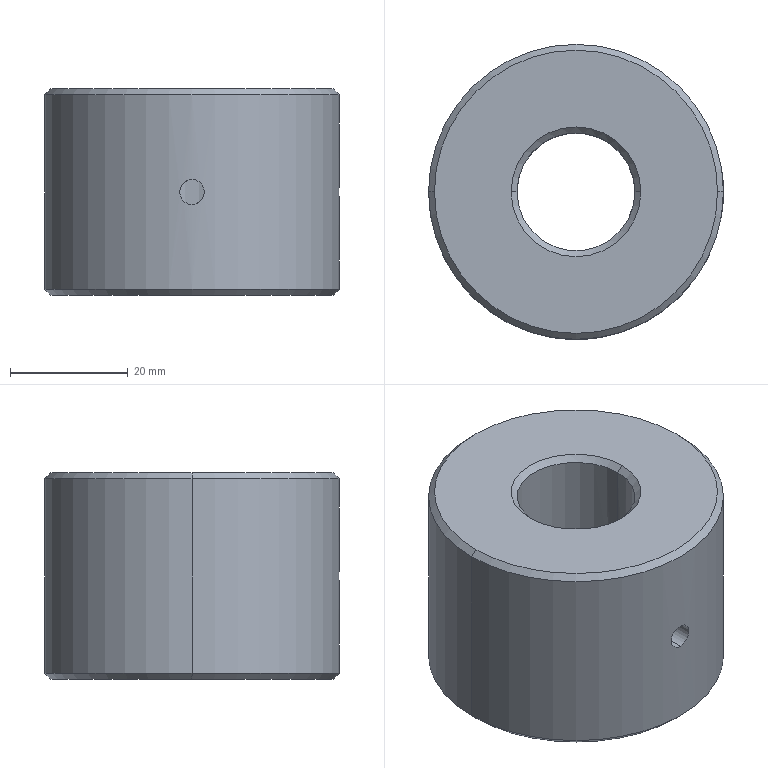Part | SolidWorks | features BaseBody 1 | 1 solid | 18 faces | box 50 x 50 x 35 mm | volume 57090 mm3 | cylinder 8 | cone 8 | plane 2 | commonest cylinder face diameters 4.2 x4 20 x2 50 x2
STEP:
#1=CARTESIAN_POINT('',(0.,-10.,15.4));
#2=VERTEX_POINT('',#1);
#3=CARTESIAN_POINT('',(0.,-10.,19.6));
#4=VERTEX_POINT('',#3);
#5=CARTESIAN_POINT('',(0.,-10.,15.4));
#6=CARTESIAN_POINT('',(-0.1391,-10.,15.4));
#7=CARTESIAN_POINT('',(-0.2759,-9.997,15.414));
#8=CARTESIAN_POINT('',(-0.5447,-9.986,15.467));
#9=CARTESIAN_POINT('',(-0.6783,-9.978,15.508));
#10=CARTESIAN_POINT('',(-0.9324,-9.957,15.613));
#11=CARTESIAN_POINT('',(-1.053,-9.945,15.678));
#12=CARTESIAN_POINT('',(-1.281,-9.918,15.83));
#13=CARTESIAN_POINT('',(-1.388,-9.904,15.919));
#14=CARTESIAN_POINT('',(-1.678,-9.86,16.208));
#15=CARTESIAN_POINT('',(-1.834,-9.831,16.442));
#16=CARTESIAN_POINT('',(-1.992,-9.8,16.821));
#17=CARTESIAN_POINT('',(-2.032,-9.791,16.953));
#18=CARTESIAN_POINT('',(-2.086,-9.78,17.224));
#19=CARTESIAN_POINT('',(-2.1,-9.777,17.361));
#20=CARTESIAN_POINT('',(-2.1,-9.777,17.636));
#21=CARTESIAN_POINT('',(-2.086,-9.78,17.775));
#22=CARTESIAN_POINT('',(-2.033,-9.791,18.045));
#23=CARTESIAN_POINT('',(-1.993,-9.8,18.176));
#24=CARTESIAN_POINT('',(-1.835,-9.831,18.558));
#25=CARTESIAN_POINT('',(-1.681,-9.86,18.789));
#26=CARTESIAN_POINT('',(-1.388,-9.904,19.082));
#27=CARTESIAN_POINT('',(-1.283,-9.918,19.168));
#28=CARTESIAN_POINT('',(-1.056,-9.945,19.32));
#29=CARTESIAN_POINT('',(-0.9328,-9.957,19.386));
#30=CARTESIAN_POINT('',(-0.6792,-9.978,19.492));
#31=CARTESIAN_POINT('',(-0.5483,-9.986,19.532));
#32=CARTESIAN_POINT('',(-0.2784,-9.997,19.586));
#33=CARTESIAN_POINT('',(-0.1391,-10.,19.6));
#34=CARTESIAN_POINT('',(0.,-10.,19.6));
#35=B_SPLINE_CURVE_WITH_KNOTS('',3,(#5,#6,#7,#8,#9,#10,#11,#12,#13,#14,#15,#16,#17,#18,#19,#20,#21,#22,#23,#24,#25,#26,#27,#28,#29,#30,#31,#32,#33,#34),.UNSPECIFIED.,.F.,.F.,(4,2,2,2,2,2,2,2,2,2,2,2,2,2,4),(0.,0.0004114,0.0008228,0.001234,0.001646,0.002468,0.00288,0.003291,0.003702,0.004114,0.004937,0.005348,0.005759,0.006171,0.006582),.UNSPECIFIED.);
#36=EDGE_CURVE('',#2,#4,#35,.T.);
#37=ORIENTED_EDGE('',*,*,#36,.T.);
#38=CARTESIAN_POINT('',(0.,-25.,19.6));
#39=VERTEX_POINT('',#38);
#40=CARTESIAN_POINT('',(0.,-25.,19.6));
#41=DIRECTION('',(0.,-1.,0.));
#42=VECTOR('',#41,1000.);
#43=LINE('',#40,#42);
#44=EDGE_CURVE('',#4,#39,#43,.T.);
#45=ORIENTED_EDGE('',*,*,#44,.T.);
#46=CARTESIAN_POINT('',(0.,-25.,15.4));
#47=VERTEX_POINT('',#46);
#48=CARTESIAN_POINT('',(0.,-25.,15.4));
#49=CARTESIAN_POINT('',(-0.1388,-25.,15.4));
#50=CARTESIAN_POINT('',(-0.2752,-24.999,15.414));
#51=CARTESIAN_POINT('',(-0.5437,-24.994,15.467));
#52=CARTESIAN_POINT('',(-0.6771,-24.991,15.507));
#53=CARTESIAN_POINT('',(-0.9313,-24.983,15.613));
#54=CARTESIAN_POINT('',(-1.052,-24.978,15.677));
#55=CARTESIAN_POINT('',(-1.28,-24.967,15.83));
#56=CARTESIAN_POINT('',(-1.388,-24.962,15.918));
#57=CARTESIAN_POINT('',(-1.679,-24.944,16.209));
#58=CARTESIAN_POINT('',(-1.835,-24.933,16.443));
#59=CARTESIAN_POINT('',(-2.045,-24.916,16.948));
#60=CARTESIAN_POINT('',(-2.1,-24.912,17.225));
#61=CARTESIAN_POINT('',(-2.1,-24.912,17.636));
#62=CARTESIAN_POINT('',(-2.086,-24.913,17.775));
#63=CARTESIAN_POINT('',(-2.033,-24.917,18.044));
#64=CARTESIAN_POINT('',(-1.993,-24.92,18.175));
#65=CARTESIAN_POINT('',(-1.888,-24.929,18.429));
#66=CARTESIAN_POINT('',(-1.823,-24.934,18.552));
#67=CARTESIAN_POINT('',(-1.671,-24.944,18.78));
#68=CARTESIAN_POINT('',(-1.584,-24.95,18.886));
#69=CARTESIAN_POINT('',(-1.388,-24.962,19.082));
#70=CARTESIAN_POINT('',(-1.282,-24.967,19.169));
#71=CARTESIAN_POINT('',(-1.055,-24.978,19.321));
#72=CARTESIAN_POINT('',(-0.932,-24.983,19.387));
#73=CARTESIAN_POINT('',(-0.6777,-24.991,19.492));
#74=CARTESIAN_POINT('',(-0.5468,-24.994,19.532));
#75=CARTESIAN_POINT('',(-0.2777,-24.999,19.586));
#76=CARTESIAN_POINT('',(-0.1388,-25.,19.6));
#77=CARTESIAN_POINT('',(0.,-25.,19.6));
#78=B_SPLINE_CURVE_WITH_KNOTS('',3,(#48,#49,#50,#51,#52,#53,#54,#55,#56,#57,#58,#59,#60,#61,#62,#63,#64,#65,#66,#67,#68,#69,#70,#71,#72,#73,#74,#75,#76,#77),.UNSPECIFIED.,.F.,.F.,(4,2,2,2,2,2,2,2,2,2,2,2,2,2,4),(0.,0.0004104,0.0008209,0.001231,0.001642,0.002463,0.003284,0.003694,0.004104,0.004515,0.004925,0.005336,0.005746,0.006157,0.006567),.UNSPECIFIED.);
#79=EDGE_CURVE('',#47,#39,#78,.T.);
#80=ORIENTED_EDGE('',*,*,#79,.F.);
#81=CARTESIAN_POINT('',(0.,-25.,15.4));
#82=DIRECTION('',(0.,-1.,0.));
#83=VECTOR('',#82,1000.);
#84=LINE('',#81,#83);
#85=EDGE_CURVE('',#2,#47,#84,.T.);
#86=ORIENTED_EDGE('',*,*,#85,.F.);
#87=EDGE_LOOP('',(#37,#45,#80,#86));
#88=FACE_OUTER_BOUND('',#87,.T.);
#89=CARTESIAN_POINT('',(0.,-25.,17.5));
#90=DIRECTION('',(0.,-1.,0.));
#91=DIRECTION('',(0.,0.,-1.));
#92=AXIS2_PLACEMENT_3D('',#89,#90,#91);
#93=CYLINDRICAL_SURFACE('',#92,2.1);
#94=ADVANCED_FACE('',(#88),#93,.F.);
#95=CARTESIAN_POINT('',(10.,0.,15.4));
#96=VERTEX_POINT('',#95);
#97=CARTESIAN_POINT('',(10.,0.,19.6));
#98=VERTEX_POINT('',#97);
#99=CARTESIAN_POINT('',(10.,0.,15.4));
#100=CARTESIAN_POINT('',(10.,-0.1391,15.4));
#101=CARTESIAN_POINT('',(9.997,-0.2759,15.414));
#102=CARTESIAN_POINT('',(9.986,-0.5447,15.467));
#103=CARTESIAN_POINT('',(9.978,-0.6783,15.508));
#104=CARTESIAN_POINT('',(9.957,-0.9324,15.613));
#105=CARTESIAN_POINT('',(9.945,-1.053,15.678));
#106=CARTESIAN_POINT('',(9.918,-1.281,15.83));
#107=CARTESIAN_POINT('',(9.904,-1.388,15.919));
#108=CARTESIAN_POINT('',(9.86,-1.678,16.208));
#109=CARTESIAN_POINT('',(9.831,-1.834,16.442));
#110=CARTESIAN_POINT('',(9.8,-1.992,16.821));
#111=CARTESIAN_POINT('',(9.791,-2.032,16.953));
#112=CARTESIAN_POINT('',(9.78,-2.086,17.224));
#113=CARTESIAN_POINT('',(9.777,-2.1,17.361));
#114=CARTESIAN_POINT('',(9.777,-2.1,17.636));
#115=CARTESIAN_POINT('',(9.78,-2.086,17.775));
#116=CARTESIAN_POINT('',(9.791,-2.033,18.045));
#117=CARTESIAN_POINT('',(9.8,-1.993,18.176));
#118=CARTESIAN_POINT('',(9.831,-1.835,18.558));
#119=CARTESIAN_POINT('',(9.86,-1.681,18.789));
#120=CARTESIAN_POINT('',(9.904,-1.388,19.082));
#121=CARTESIAN_POINT('',(9.918,-1.283,19.168));
#122=CARTESIAN_POINT('',(9.945,-1.056,19.32));
#123=CARTESIAN_POINT('',(9.957,-0.9328,19.386));
#124=CARTESIAN_POINT('',(9.978,-0.6792,19.492));
#125=CARTESIAN_POINT('',(9.986,-0.5483,19.532));
#126=CARTESIAN_POINT('',(9.997,-0.2784,19.586));
#127=CARTESIAN_POINT('',(10.,-0.1391,19.6));
#128=CARTESIAN_POINT('',(10.,0.,19.6));
#129=B_SPLINE_CURVE_WITH_KNOTS('',3,(#99,#100,#101,#102,#103,#104,#105,#106,#107,#108,#109,#110,#111,#112,#113,#114,#115,#116,#117,#118,#119,#120,#121,#122,#123,#124,#125,#126,#127,#128),.UNSPECIFIED.,.F.,.F.,(4,2,2,2,2,2,2,2,2,2,2,2,2,2,4),(0.,0.0004114,0.0008228,0.001234,0.001646,0.002468,0.00288,0.003291,0.003702,0.004114,0.004937,0.005348,0.005759,0.006171,0.006582),.UNSPECIFIED.);
#130=EDGE_CURVE('',#96,#98,#129,.T.);
#131=ORIENTED_EDGE('',*,*,#130,.T.);
#132=CARTESIAN_POINT('',(25.,0.,19.6));
#133=VERTEX_POINT('',#132);
#134=CARTESIAN_POINT('',(25.,0.,19.6));
#135=DIRECTION('',(1.,0.,0.));
#136=VECTOR('',#135,1000.);
#137=LINE('',#134,#136);
#138=EDGE_CURVE('',#98,#133,#137,.T.);
#139=ORIENTED_EDGE('',*,*,#138,.T.);
#140=CARTESIAN_POINT('',(25.,0.,15.4));
#141=VERTEX_POINT('',#140);
#142=CARTESIAN_POINT('',(25.,0.,15.4));
#143=CARTESIAN_POINT('',(25.,-0.1388,15.4));
#144=CARTESIAN_POINT('',(24.999,-0.2752,15.414));
#145=CARTESIAN_POINT('',(24.994,-0.5437,15.467));
#146=CARTESIAN_POINT('',(24.991,-0.6771,15.507));
#147=CARTESIAN_POINT('',(24.983,-0.9313,15.613));
#148=CARTESIAN_POINT('',(24.978,-1.052,15.677));
#149=CARTESIAN_POINT('',(24.967,-1.28,15.83));
#150=CARTESIAN_POINT('',(24.962,-1.388,15.918));
#151=CARTESIAN_POINT('',(24.944,-1.679,16.209));
#152=CARTESIAN_POINT('',(24.933,-1.835,16.443));
#153=CARTESIAN_POINT('',(24.916,-2.045,16.948));
#154=CARTESIAN_POINT('',(24.912,-2.1,17.225));
#155=CARTESIAN_POINT('',(24.912,-2.1,17.636));
#156=CARTESIAN_POINT('',(24.913,-2.086,17.775));
#157=CARTESIAN_POINT('',(24.917,-2.033,18.044));
#158=CARTESIAN_POINT('',(24.92,-1.993,18.175));
#159=CARTESIAN_POINT('',(24.929,-1.888,18.429));
#160=CARTESIAN_POINT('',(24.934,-1.823,18.552));
#161=CARTESIAN_POINT('',(24.944,-1.671,18.78));
#162=CARTESIAN_POINT('',(24.95,-1.584,18.886));
#163=CARTESIAN_POINT('',(24.962,-1.388,19.082));
#164=CARTESIAN_POINT('',(24.967,-1.282,19.169));
#165=CARTESIAN_POINT('',(24.978,-1.055,19.321));
#166=CARTESIAN_POINT('',(24.983,-0.932,19.387));
#167=CARTESIAN_POINT('',(24.991,-0.6777,19.492));
#168=CARTESIAN_POINT('',(24.994,-0.5468,19.532));
#169=CARTESIAN_POINT('',(24.999,-0.2777,19.586));
#170=CARTESIAN_POINT('',(25.,-0.1388,19.6));
#171=CARTESIAN_POINT('',(25.,0.,19.6));
#172=B_SPLINE_CURVE_WITH_KNOTS('',3,(#142,#143,#144,#145,#146,#147,#148,#149,#150,#151,#152,#153,#154,#155,#156,#157,#158,#159,#160,#161,#162,#163,#164,#165,#166,#167,#168,#169,#170,#171),.UNSPECIFIED.,.F.,.F.,(4,2,2,2,2,2,2,2,2,2,2,2,2,2,4),(0.,0.0004104,0.0008209,0.001231,0.001642,0.002463,0.003284,0.003694,0.004104,0.004515,0.004925,0.005336,0.005746,0.006157,0.006567),.UNSPECIFIED.);
#173=EDGE_CURVE('',#141,#133,#172,.T.);
#174=ORIENTED_EDGE('',*,*,#173,.F.);
#175=CARTESIAN_POINT('',(25.,0.,15.4));
#176=DIRECTION('',(1.,0.,0.));
#177=VECTOR('',#176,1000.);
#178=LINE('',#175,#177);
#179=EDGE_CURVE('',#96,#141,#178,.T.);
#180=ORIENTED_EDGE('',*,*,#179,.F.);
#181=EDGE_LOOP('',(#131,#139,#174,#180));
#182=FACE_OUTER_BOUND('',#181,.T.);
#183=CARTESIAN_POINT('',(25.,0.,17.5));
#184=DIRECTION('',(1.,0.,0.));
#185=DIRECTION('',(0.,0.,-1.));
#186=AXIS2_PLACEMENT_3D('',#183,#184,#185);
#187=CYLINDRICAL_SURFACE('',#186,2.1);
#188=ADVANCED_FACE('',(#182),#187,.F.);
#189=CARTESIAN_POINT('',(10.,0.,1.));
#190=VERTEX_POINT('',#189);
#191=CARTESIAN_POINT('',(-10.,0.,1.));
#192=VERTEX_POINT('',#191);
#193=CARTESIAN_POINT('',(0.,0.,1.));
#194=DIRECTION('',(0.,0.,-1.));
#195=DIRECTION('',(1.,0.,0.));
#196=AXIS2_PLACEMENT_3D('',#193,#194,#195);
#197=CIRCLE('',#196,10.);
#198=EDGE_CURVE('',#190,#192,#197,.T.);
#199=ORIENTED_EDGE('',*,*,#198,.F.);
#200=CARTESIAN_POINT('',(11.,0.,0.));
#201=VERTEX_POINT('',#200);
#202=CARTESIAN_POINT('',(11.,0.,0.));
#203=DIRECTION('',(0.7071,0.,-0.7071));
#204=VECTOR('',#203,1000.);
#205=LINE('',#202,#204);
#206=EDGE_CURVE('',#190,#201,#205,.T.);
#207=ORIENTED_EDGE('',*,*,#206,.T.);
#208=CARTESIAN_POINT('',(-11.,0.,0.));
#209=VERTEX_POINT('',#208);
#210=CARTESIAN_POINT('',(0.,0.,0.));
#211=DIRECTION('',(0.,0.,1.));
#212=DIRECTION('',(1.,0.,0.));
#213=AXIS2_PLACEMENT_3D('',#210,#211,#212);
#214=CIRCLE('',#213,11.);
#215=EDGE_CURVE('',#209,#201,#214,.T.);
#216=ORIENTED_EDGE('',*,*,#215,.F.);
#217=CARTESIAN_POINT('',(-11.,0.,0.));
#218=DIRECTION('',(-0.7071,0.,-0.7071));
#219=VECTOR('',#218,1000.);
#220=LINE('',#217,#219);
#221=EDGE_CURVE('',#192,#209,#220,.T.);
#222=ORIENTED_EDGE('',*,*,#221,.F.);
#223=EDGE_LOOP('',(#199,#207,#216,#222));
#224=FACE_OUTER_BOUND('',#223,.T.);
#225=CARTESIAN_POINT('',(0.,0.,0.));
#226=DIRECTION('',(0.,0.,-1.));
#227=DIRECTION('',(-1.,0.,0.));
#228=AXIS2_PLACEMENT_3D('',#225,#226,#227);
#229=CONICAL_SURFACE('',#228,11.,0.7854);
#230=ADVANCED_FACE('',(#224),#229,.F.);
#231=CARTESIAN_POINT('',(-10.,0.,34.));
#232=VERTEX_POINT('',#231);
#233=CARTESIAN_POINT('',(10.,0.,34.));
#234=VERTEX_POINT('',#233);
#235=CARTESIAN_POINT('',(0.,0.,34.));
#236=DIRECTION('',(0.,0.,1.));
#237=DIRECTION('',(1.,0.,0.));
#238=AXIS2_PLACEMENT_3D('',#235,#236,#237);
#239=CIRCLE('',#238,10.);
#240=EDGE_CURVE('',#232,#234,#239,.T.);
#241=ORIENTED_EDGE('',*,*,#240,.F.);
#242=CARTESIAN_POINT('',(-11.,0.,35.));
#243=VERTEX_POINT('',#242);
#244=CARTESIAN_POINT('',(-10.,0.,34.));
#245=DIRECTION('',(-0.7071,0.,0.7071));
#246=VECTOR('',#245,1000.);
#247=LINE('',#244,#246);
#248=EDGE_CURVE('',#232,#243,#247,.T.);
#249=ORIENTED_EDGE('',*,*,#248,.T.);
#250=CARTESIAN_POINT('',(11.,0.,35.));
#251=VERTEX_POINT('',#250);
#252=CARTESIAN_POINT('',(0.,0.,35.));
#253=DIRECTION('',(0.,0.,-1.));
#254=DIRECTION('',(1.,0.,0.));
#255=AXIS2_PLACEMENT_3D('',#252,#253,#254);
#256=CIRCLE('',#255,11.);
#257=EDGE_CURVE('',#251,#243,#256,.T.);
#258=ORIENTED_EDGE('',*,*,#257,.F.);
#259=CARTESIAN_POINT('',(10.,0.,34.));
#260=DIRECTION('',(0.7071,0.,0.7071));
#261=VECTOR('',#260,1000.);
#262=LINE('',#259,#261);
#263=EDGE_CURVE('',#234,#251,#262,.T.);
#264=ORIENTED_EDGE('',*,*,#263,.F.);
#265=EDGE_LOOP('',(#241,#249,#258,#264));
#266=FACE_OUTER_BOUND('',#265,.T.);
#267=CARTESIAN_POINT('',(0.,0.,34.));
#268=DIRECTION('',(0.,0.,1.));
#269=DIRECTION('',(1.,0.,0.));
#270=AXIS2_PLACEMENT_3D('',#267,#268,#269);
#271=CONICAL_SURFACE('',#270,10.,0.7854);
#272=ADVANCED_FACE('',(#266),#271,.F.);
#273=CARTESIAN_POINT('',(24.,0.,35.));
#274=VERTEX_POINT('',#273);
#275=CARTESIAN_POINT('',(-24.,0.,35.));
#276=VERTEX_POINT('',#275);
#277=CARTESIAN_POINT('',(0.,0.,35.));
#278=DIRECTION('',(0.,0.,1.));
#279=DIRECTION('',(1.,0.,0.));
#280=AXIS2_PLACEMENT_3D('',#277,#278,#279);
#281=CIRCLE('',#280,24.);
#282=EDGE_CURVE('',#274,#276,#281,.T.);
#283=ORIENTED_EDGE('',*,*,#282,.F.);
#284=CARTESIAN_POINT('',(25.,0.,34.));
#285=VERTEX_POINT('',#284);
#286=CARTESIAN_POINT('',(24.,0.,35.));
#287=DIRECTION('',(0.7071,0.,-0.7071));
#288=VECTOR('',#287,1000.);
#289=LINE('',#286,#288);
#290=EDGE_CURVE('',#274,#285,#289,.T.);
#291=ORIENTED_EDGE('',*,*,#290,.T.);
#292=CARTESIAN_POINT('',(-25.,0.,34.));
#293=VERTEX_POINT('',#292);
#294=CARTESIAN_POINT('',(0.,0.,34.));
#295=DIRECTION('',(0.,0.,-1.));
#296=DIRECTION('',(1.,0.,0.));
#297=AXIS2_PLACEMENT_3D('',#294,#295,#296);
#298=CIRCLE('',#297,25.);
#299=EDGE_CURVE('',#293,#285,#298,.T.);
#300=ORIENTED_EDGE('',*,*,#299,.F.);
#301=CARTESIAN_POINT('',(-24.,0.,35.));
#302=DIRECTION('',(-0.7071,0.,-0.7071));
#303=VECTOR('',#302,1000.);
#304=LINE('',#301,#303);
#305=EDGE_CURVE('',#276,#293,#304,.T.);
#306=ORIENTED_EDGE('',*,*,#305,.F.);
#307=EDGE_LOOP('',(#283,#291,#300,#306));
#308=FACE_OUTER_BOUND('',#307,.T.);
#309=CARTESIAN_POINT('',(0.,0.,35.));
#310=DIRECTION('',(0.,0.,-1.));
#311=DIRECTION('',(-1.,0.,0.));
#312=AXIS2_PLACEMENT_3D('',#309,#310,#311);
#313=CONICAL_SURFACE('',#312,24.,0.7854);
#314=ADVANCED_FACE('',(#308),#313,.T.);
#315=CARTESIAN_POINT('',(-24.,0.,0.));
#316=VERTEX_POINT('',#315);
#317=CARTESIAN_POINT('',(24.,0.,0.));
#318=VERTEX_POINT('',#317);
#319=CARTESIAN_POINT('',(0.,0.,0.));
#320=DIRECTION('',(0.,0.,-1.));
#321=DIRECTION('',(1.,0.,0.));
#322=AXIS2_PLACEMENT_3D('',#319,#320,#321);
#323=CIRCLE('',#322,24.);
#324=EDGE_CURVE('',#316,#318,#323,.T.);
#325=ORIENTED_EDGE('',*,*,#324,.F.);
#326=CARTESIAN_POINT('',(-25.,0.,1.));
#327=VERTEX_POINT('',#326);
#328=CARTESIAN_POINT('',(-25.,0.,1.));
#329=DIRECTION('',(-0.7071,0.,0.7071));
#330=VECTOR('',#329,1000.);
#331=LINE('',#328,#330);
#332=EDGE_CURVE('',#316,#327,#331,.T.);
#333=ORIENTED_EDGE('',*,*,#332,.T.);
#334=CARTESIAN_POINT('',(25.,0.,1.));
#335=VERTEX_POINT('',#334);
#336=CARTESIAN_POINT('',(0.,0.,1.));
#337=DIRECTION('',(0.,0.,1.));
#338=DIRECTION('',(1.,0.,0.));
#339=AXIS2_PLACEMENT_3D('',#336,#337,#338);
#340=CIRCLE('',#339,25.);
#341=EDGE_CURVE('',#335,#327,#340,.T.);
#342=ORIENTED_EDGE('',*,*,#341,.F.);
#343=CARTESIAN_POINT('',(25.,0.,1.));
#344=DIRECTION('',(0.7071,0.,0.7071));
#345=VECTOR('',#344,1000.);
#346=LINE('',#343,#345);
#347=EDGE_CURVE('',#318,#335,#346,.T.);
#348=ORIENTED_EDGE('',*,*,#347,.F.);
#349=EDGE_LOOP('',(#325,#333,#342,#348));
#350=FACE_OUTER_BOUND('',#349,.T.);
#351=CARTESIAN_POINT('',(0.,0.,1.));
#352=DIRECTION('',(0.,0.,1.));
#353=DIRECTION('',(1.,0.,0.));
#354=AXIS2_PLACEMENT_3D('',#351,#352,#353);
#355=CONICAL_SURFACE('',#354,25.,0.7854);
#356=ADVANCED_FACE('',(#350),#355,.T.);
#357=ORIENTED_EDGE('',*,*,#36,.F.);
#358=CARTESIAN_POINT('',(0.,-10.,19.6));
#359=CARTESIAN_POINT('',(0.1391,-10.,19.6));
#360=CARTESIAN_POINT('',(0.2759,-9.997,19.586));
#361=CARTESIAN_POINT('',(0.5447,-9.986,19.533));
#362=CARTESIAN_POINT('',(0.6783,-9.978,19.492));
#363=CARTESIAN_POINT('',(0.9324,-9.957,19.387));
#364=CARTESIAN_POINT('',(1.053,-9.945,19.322));
#365=CARTESIAN_POINT('',(1.281,-9.918,19.17));
#366=CARTESIAN_POINT('',(1.388,-9.904,19.081));
#367=CARTESIAN_POINT('',(1.678,-9.86,18.792));
#368=CARTESIAN_POINT('',(1.834,-9.831,18.558));
#369=CARTESIAN_POINT('',(1.992,-9.8,18.179));
#370=CARTESIAN_POINT('',(2.032,-9.791,18.047));
#371=CARTESIAN_POINT('',(2.086,-9.78,17.776));
#372=CARTESIAN_POINT('',(2.1,-9.777,17.639));
#373=CARTESIAN_POINT('',(2.1,-9.777,17.364));
#374=CARTESIAN_POINT('',(2.086,-9.78,17.225));
#375=CARTESIAN_POINT('',(2.033,-9.791,16.955));
#376=CARTESIAN_POINT('',(1.993,-9.8,16.824));
#377=CARTESIAN_POINT('',(1.835,-9.831,16.442));
#378=CARTESIAN_POINT('',(1.681,-9.86,16.211));
#379=CARTESIAN_POINT('',(1.388,-9.904,15.918));
#380=CARTESIAN_POINT('',(1.283,-9.918,15.832));
#381=CARTESIAN_POINT('',(1.056,-9.945,15.68));
#382=CARTESIAN_POINT('',(0.9328,-9.957,15.614));
#383=CARTESIAN_POINT('',(0.6792,-9.978,15.508));
#384=CARTESIAN_POINT('',(0.5483,-9.986,15.468));
#385=CARTESIAN_POINT('',(0.2784,-9.997,15.414));
#386=CARTESIAN_POINT('',(0.1391,-10.,15.4));
#387=CARTESIAN_POINT('',(0.,-10.,15.4));
#388=B_SPLINE_CURVE_WITH_KNOTS('',3,(#358,#359,#360,#361,#362,#363,#364,#365,#366,#367,#368,#369,#370,#371,#372,#373,#374,#375,#376,#377,#378,#379,#380,#381,#382,#383,#384,#385,#386,#387),.UNSPECIFIED.,.F.,.F.,(4,2,2,2,2,2,2,2,2,2,2,2,2,2,4),(0.006582,0.006993,0.007405,0.007816,0.008228,0.00905,0.009462,0.009873,0.01028,0.0107,0.01152,0.01193,0.01234,0.01275,0.01316),.UNSPECIFIED.);
#389=EDGE_CURVE('',#4,#2,#388,.T.);
#390=ORIENTED_EDGE('',*,*,#389,.F.);
#391=EDGE_LOOP('',(#357,#390));
#392=FACE_BOUND('',#391,.T.);
#393=ORIENTED_EDGE('',*,*,#240,.T.);
#394=CARTESIAN_POINT('',(10.,0.,35.));
#395=DIRECTION('',(0.,0.,-1.));
#396=VECTOR('',#395,1000.);
#397=LINE('',#394,#396);
#398=EDGE_CURVE('',#234,#98,#397,.T.);
#399=ORIENTED_EDGE('',*,*,#398,.T.);
#400=ORIENTED_EDGE('',*,*,#130,.F.);
#401=CARTESIAN_POINT('',(10.,0.,35.));
#402=DIRECTION('',(0.,0.,-1.));
#403=VECTOR('',#402,1000.);
#404=LINE('',#401,#403);
#405=EDGE_CURVE('',#96,#190,#404,.T.);
#406=ORIENTED_EDGE('',*,*,#405,.T.);
#407=ORIENTED_EDGE('',*,*,#198,.T.);
#408=CARTESIAN_POINT('',(-10.,0.,35.));
#409=DIRECTION('',(0.,0.,-1.));
#410=VECTOR('',#409,1000.);
#411=LINE('',#408,#410);
#412=EDGE_CURVE('',#232,#192,#411,.T.);
#413=ORIENTED_EDGE('',*,*,#412,.F.);
#414=EDGE_LOOP('',(#393,#399,#400,#406,#407,#413));
#415=FACE_OUTER_BOUND('',#414,.T.);
#416=CARTESIAN_POINT('',(0.,0.,35.));
#417=DIRECTION('',(0.,0.,-1.));
#418=DIRECTION('',(-1.,0.,0.));
#419=AXIS2_PLACEMENT_3D('',#416,#417,#418);
#420=CYLINDRICAL_SURFACE('',#419,10.);
#421=ADVANCED_FACE('',(#392,#415),#420,.F.);
#422=ORIENTED_EDGE('',*,*,#299,.T.);
#423=CARTESIAN_POINT('',(25.,0.,35.));
#424=DIRECTION('',(0.,0.,-1.));
#425=VECTOR('',#424,1000.);
#426=LINE('',#423,#425);
#427=EDGE_CURVE('',#285,#133,#426,.T.);
#428=ORIENTED_EDGE('',*,*,#427,.T.);
#429=CARTESIAN_POINT('',(25.,0.,19.6));
#430=CARTESIAN_POINT('',(25.,0.1388,19.6));
#431=CARTESIAN_POINT('',(24.999,0.2752,19.586));
#432=CARTESIAN_POINT('',(24.994,0.5437,19.533));
#433=CARTESIAN_POINT('',(24.991,0.6771,19.493));
#434=CARTESIAN_POINT('',(24.983,0.9313,19.387));
#435=CARTESIAN_POINT('',(24.978,1.052,19.323));
#436=CARTESIAN_POINT('',(24.967,1.28,19.17));
#437=CARTESIAN_POINT('',(24.962,1.388,19.082));
#438=CARTESIAN_POINT('',(24.944,1.679,18.791));
#439=CARTESIAN_POINT('',(24.933,1.835,18.557));
#440=CARTESIAN_POINT('',(24.916,2.045,18.052));
#441=CARTESIAN_POINT('',(24.912,2.1,17.775));
#442=CARTESIAN_POINT('',(24.912,2.1,17.364));
#443=CARTESIAN_POINT('',(24.913,2.086,17.225));
#444=CARTESIAN_POINT('',(24.917,2.033,16.956));
#445=CARTESIAN_POINT('',(24.92,1.993,16.825));
#446=CARTESIAN_POINT('',(24.929,1.888,16.571));
#447=CARTESIAN_POINT('',(24.934,1.823,16.448));
#448=CARTESIAN_POINT('',(24.944,1.671,16.22));
#449=CARTESIAN_POINT('',(24.95,1.584,16.114));
#450=CARTESIAN_POINT('',(24.962,1.388,15.918));
#451=CARTESIAN_POINT('',(24.967,1.282,15.831));
#452=CARTESIAN_POINT('',(24.978,1.055,15.679));
#453=CARTESIAN_POINT('',(24.983,0.932,15.613));
#454=CARTESIAN_POINT('',(24.991,0.6777,15.508));
#455=CARTESIAN_POINT('',(24.994,0.5468,15.468));
#456=CARTESIAN_POINT('',(24.999,0.2777,15.414));
#457=CARTESIAN_POINT('',(25.,0.1388,15.4));
#458=CARTESIAN_POINT('',(25.,0.,15.4));
#459=B_SPLINE_CURVE_WITH_KNOTS('',3,(#429,#430,#431,#432,#433,#434,#435,#436,#437,#438,#439,#440,#441,#442,#443,#444,#445,#446,#447,#448,#449,#450,#451,#452,#453,#454,#455,#456,#457,#458),.UNSPECIFIED.,.F.,.F.,(4,2,2,2,2,2,2,2,2,2,2,2,2,2,4),(0.006567,0.006977,0.007388,0.007798,0.008209,0.00903,0.009851,0.01026,0.01067,0.01108,0.01149,0.0119,0.01231,0.01272,0.01313),.UNSPECIFIED.);
#460=EDGE_CURVE('',#133,#141,#459,.T.);
#461=ORIENTED_EDGE('',*,*,#460,.T.);
#462=CARTESIAN_POINT('',(25.,0.,35.));
#463=DIRECTION('',(0.,0.,-1.));
#464=VECTOR('',#463,1000.);
#465=LINE('',#462,#464);
#466=EDGE_CURVE('',#141,#335,#465,.T.);
#467=ORIENTED_EDGE('',*,*,#466,.T.);
#468=ORIENTED_EDGE('',*,*,#341,.T.);
#469=CARTESIAN_POINT('',(-25.,0.,35.));
#470=DIRECTION('',(0.,0.,-1.));
#471=VECTOR('',#470,1000.);
#472=LINE('',#469,#471);
#473=EDGE_CURVE('',#293,#327,#472,.T.);
#474=ORIENTED_EDGE('',*,*,#473,.F.);
#475=EDGE_LOOP('',(#422,#428,#461,#467,#468,#474));
#476=FACE_OUTER_BOUND('',#475,.T.);
#477=CARTESIAN_POINT('',(0.,0.,35.));
#478=DIRECTION('',(0.,0.,-1.));
#479=DIRECTION('',(-1.,0.,0.));
#480=AXIS2_PLACEMENT_3D('',#477,#478,#479);
#481=CYLINDRICAL_SURFACE('',#480,25.);
#482=ADVANCED_FACE('',(#476),#481,.T.);
#483=ORIENTED_EDGE('',*,*,#215,.T.);
#484=CARTESIAN_POINT('',(0.,0.,0.));
#485=DIRECTION('',(0.,0.,1.));
#486=DIRECTION('',(1.,0.,0.));
#487=AXIS2_PLACEMENT_3D('',#484,#485,#486);
#488=CIRCLE('',#487,11.);
#489=EDGE_CURVE('',#201,#209,#488,.T.);
#490=ORIENTED_EDGE('',*,*,#489,.T.);
#491=EDGE_LOOP('',(#483,#490));
#492=FACE_BOUND('',#491,.T.);
#493=CARTESIAN_POINT('',(0.,0.,0.));
#494=DIRECTION('',(0.,0.,-1.));
#495=DIRECTION('',(1.,0.,0.));
#496=AXIS2_PLACEMENT_3D('',#493,#494,#495);
#497=CIRCLE('',#496,24.);
#498=EDGE_CURVE('',#318,#316,#497,.T.);
#499=ORIENTED_EDGE('',*,*,#498,.T.);
#500=ORIENTED_EDGE('',*,*,#324,.T.);
#501=EDGE_LOOP('',(#499,#500));
#502=FACE_OUTER_BOUND('',#501,.T.);
#503=CARTESIAN_POINT('',(0.,0.,0.));
#504=DIRECTION('',(0.,0.,1.));
#505=DIRECTION('',(1.,0.,0.));
#506=AXIS2_PLACEMENT_3D('',#503,#504,#505);
#507=PLANE('',#506);
#508=ADVANCED_FACE('',(#492,#502),#507,.F.);
#509=ORIENTED_EDGE('',*,*,#257,.T.);
#510=CARTESIAN_POINT('',(0.,0.,35.));
#511=DIRECTION('',(0.,0.,-1.));
#512=DIRECTION('',(1.,0.,0.));
#513=AXIS2_PLACEMENT_3D('',#510,#511,#512);
#514=CIRCLE('',#513,11.);
#515=EDGE_CURVE('',#243,#251,#514,.T.);
#516=ORIENTED_EDGE('',*,*,#515,.T.);
#517=EDGE_LOOP('',(#509,#516));
#518=FACE_BOUND('',#517,.T.);
#519=CARTESIAN_POINT('',(0.,0.,35.));
#520=DIRECTION('',(0.,0.,1.));
#521=DIRECTION('',(1.,0.,0.));
#522=AXIS2_PLACEMENT_3D('',#519,#520,#521);
#523=CIRCLE('',#522,24.);
#524=EDGE_CURVE('',#276,#274,#523,.T.);
#525=ORIENTED_EDGE('',*,*,#524,.T.);
#526=ORIENTED_EDGE('',*,*,#282,.T.);
#527=EDGE_LOOP('',(#525,#526));
#528=FACE_OUTER_BOUND('',#527,.T.);
#529=CARTESIAN_POINT('',(0.,0.,35.));
#530=DIRECTION('',(0.,0.,1.));
#531=DIRECTION('',(1.,0.,0.));
#532=AXIS2_PLACEMENT_3D('',#529,#530,#531);
#533=PLANE('',#532);
#534=ADVANCED_FACE('',(#518,#528),#533,.T.);
#535=ORIENTED_EDGE('',*,*,#427,.F.);
#536=CARTESIAN_POINT('',(0.,0.,34.));
#537=DIRECTION('',(0.,0.,-1.));
#538=DIRECTION('',(1.,0.,0.));
#539=AXIS2_PLACEMENT_3D('',#536,#537,#538);
#540=CIRCLE('',#539,25.);
#541=EDGE_CURVE('',#285,#293,#540,.T.);
#542=ORIENTED_EDGE('',*,*,#541,.T.);
#543=ORIENTED_EDGE('',*,*,#473,.T.);
#544=CARTESIAN_POINT('',(0.,0.,1.));
#545=DIRECTION('',(0.,0.,1.));
#546=DIRECTION('',(1.,0.,0.));
#547=AXIS2_PLACEMENT_3D('',#544,#545,#546);
#548=CIRCLE('',#547,25.);
#549=EDGE_CURVE('',#327,#335,#548,.T.);
#550=ORIENTED_EDGE('',*,*,#549,.T.);
#551=ORIENTED_EDGE('',*,*,#466,.F.);
#552=ORIENTED_EDGE('',*,*,#173,.T.);
#553=EDGE_LOOP('',(#535,#542,#543,#550,#551,#552));
#554=FACE_OUTER_BOUND('',#553,.T.);
#555=ORIENTED_EDGE('',*,*,#79,.T.);
#556=CARTESIAN_POINT('',(0.,-25.,19.6));
#557=CARTESIAN_POINT('',(0.1388,-25.,19.6));
#558=CARTESIAN_POINT('',(0.2752,-24.999,19.586));
#559=CARTESIAN_POINT('',(0.5437,-24.994,19.533));
#560=CARTESIAN_POINT('',(0.6771,-24.991,19.493));
#561=CARTESIAN_POINT('',(0.9313,-24.983,19.387));
#562=CARTESIAN_POINT('',(1.052,-24.978,19.323));
#563=CARTESIAN_POINT('',(1.28,-24.967,19.17));
#564=CARTESIAN_POINT('',(1.388,-24.962,19.082));
#565=CARTESIAN_POINT('',(1.679,-24.944,18.791));
#566=CARTESIAN_POINT('',(1.835,-24.933,18.557));
#567=CARTESIAN_POINT('',(2.045,-24.916,18.052));
#568=CARTESIAN_POINT('',(2.1,-24.912,17.775));
#569=CARTESIAN_POINT('',(2.1,-24.912,17.364));
#570=CARTESIAN_POINT('',(2.086,-24.913,17.225));
#571=CARTESIAN_POINT('',(2.033,-24.917,16.956));
#572=CARTESIAN_POINT('',(1.993,-24.92,16.825));
#573=CARTESIAN_POINT('',(1.888,-24.929,16.571));
#574=CARTESIAN_POINT('',(1.823,-24.934,16.448));
#575=CARTESIAN_POINT('',(1.671,-24.944,16.22));
#576=CARTESIAN_POINT('',(1.584,-24.95,16.114));
#577=CARTESIAN_POINT('',(1.388,-24.962,15.918));
#578=CARTESIAN_POINT('',(1.282,-24.967,15.831));
#579=CARTESIAN_POINT('',(1.055,-24.978,15.679));
#580=CARTESIAN_POINT('',(0.932,-24.983,15.613));
#581=CARTESIAN_POINT('',(0.6777,-24.991,15.508));
#582=CARTESIAN_POINT('',(0.5468,-24.994,15.468));
#583=CARTESIAN_POINT('',(0.2777,-24.999,15.414));
#584=CARTESIAN_POINT('',(0.1388,-25.,15.4));
#585=CARTESIAN_POINT('',(0.,-25.,15.4));
#586=B_SPLINE_CURVE_WITH_KNOTS('',3,(#556,#557,#558,#559,#560,#561,#562,#563,#564,#565,#566,#567,#568,#569,#570,#571,#572,#573,#574,#575,#576,#577,#578,#579,#580,#581,#582,#583,#584,#585),.UNSPECIFIED.,.F.,.F.,(4,2,2,2,2,2,2,2,2,2,2,2,2,2,4),(0.006567,0.006977,0.007388,0.007798,0.008209,0.00903,0.009851,0.01026,0.01067,0.01108,0.01149,0.0119,0.01231,0.01272,0.01313),.UNSPECIFIED.);
#587=EDGE_CURVE('',#39,#47,#586,.T.);
#588=ORIENTED_EDGE('',*,*,#587,.T.);
#589=EDGE_LOOP('',(#555,#588));
#590=FACE_BOUND('',#589,.T.);
#591=CARTESIAN_POINT('',(0.,0.,35.));
#592=DIRECTION('',(0.,0.,-1.));
#593=DIRECTION('',(-1.,0.,0.));
#594=AXIS2_PLACEMENT_3D('',#591,#592,#593);
#595=CYLINDRICAL_SURFACE('',#594,25.);
#596=ADVANCED_FACE('',(#554,#590),#595,.T.);
#597=ORIENTED_EDGE('',*,*,#398,.F.);
#598=CARTESIAN_POINT('',(0.,0.,34.));
#599=DIRECTION('',(0.,0.,1.));
#600=DIRECTION('',(1.,0.,0.));
#601=AXIS2_PLACEMENT_3D('',#598,#599,#600);
#602=CIRCLE('',#601,10.);
#603=EDGE_CURVE('',#234,#232,#602,.T.);
#604=ORIENTED_EDGE('',*,*,#603,.T.);
#605=ORIENTED_EDGE('',*,*,#412,.T.);
#606=CARTESIAN_POINT('',(0.,0.,1.));
#607=DIRECTION('',(0.,0.,-1.));
#608=DIRECTION('',(1.,0.,0.));
#609=AXIS2_PLACEMENT_3D('',#606,#607,#608);
#610=CIRCLE('',#609,10.);
#611=EDGE_CURVE('',#192,#190,#610,.T.);
#612=ORIENTED_EDGE('',*,*,#611,.T.);
#613=ORIENTED_EDGE('',*,*,#405,.F.);
#614=CARTESIAN_POINT('',(10.,0.,19.6));
#615=CARTESIAN_POINT('',(10.,0.1391,19.6));
#616=CARTESIAN_POINT('',(9.997,0.2759,19.586));
#617=CARTESIAN_POINT('',(9.986,0.5447,19.533));
#618=CARTESIAN_POINT('',(9.978,0.6783,19.492));
#619=CARTESIAN_POINT('',(9.957,0.9324,19.387));
#620=CARTESIAN_POINT('',(9.945,1.053,19.322));
#621=CARTESIAN_POINT('',(9.918,1.281,19.17));
#622=CARTESIAN_POINT('',(9.904,1.388,19.081));
#623=CARTESIAN_POINT('',(9.86,1.678,18.792));
#624=CARTESIAN_POINT('',(9.831,1.834,18.558));
#625=CARTESIAN_POINT('',(9.8,1.992,18.179));
#626=CARTESIAN_POINT('',(9.791,2.032,18.047));
#627=CARTESIAN_POINT('',(9.78,2.086,17.776));
#628=CARTESIAN_POINT('',(9.777,2.1,17.639));
#629=CARTESIAN_POINT('',(9.777,2.1,17.364));
#630=CARTESIAN_POINT('',(9.78,2.086,17.225));
#631=CARTESIAN_POINT('',(9.791,2.033,16.955));
#632=CARTESIAN_POINT('',(9.8,1.993,16.824));
#633=CARTESIAN_POINT('',(9.831,1.835,16.442));
#634=CARTESIAN_POINT('',(9.86,1.681,16.211));
#635=CARTESIAN_POINT('',(9.904,1.388,15.918));
#636=CARTESIAN_POINT('',(9.918,1.283,15.832));
#637=CARTESIAN_POINT('',(9.945,1.056,15.68));
#638=CARTESIAN_POINT('',(9.957,0.9328,15.614));
#639=CARTESIAN_POINT('',(9.978,0.6792,15.508));
#640=CARTESIAN_POINT('',(9.986,0.5483,15.468));
#641=CARTESIAN_POINT('',(9.997,0.2784,15.414));
#642=CARTESIAN_POINT('',(10.,0.1391,15.4));
#643=CARTESIAN_POINT('',(10.,0.,15.4));
#644=B_SPLINE_CURVE_WITH_KNOTS('',3,(#614,#615,#616,#617,#618,#619,#620,#621,#622,#623,#624,#625,#626,#627,#628,#629,#630,#631,#632,#633,#634,#635,#636,#637,#638,#639,#640,#641,#642,#643),.UNSPECIFIED.,.F.,.F.,(4,2,2,2,2,2,2,2,2,2,2,2,2,2,4),(0.006582,0.006993,0.007405,0.007816,0.008228,0.00905,0.009462,0.009873,0.01028,0.0107,0.01152,0.01193,0.01234,0.01275,0.01316),.UNSPECIFIED.);
#645=EDGE_CURVE('',#98,#96,#644,.T.);
#646=ORIENTED_EDGE('',*,*,#645,.F.);
#647=EDGE_LOOP('',(#597,#604,#605,#612,#613,#646));
#648=FACE_OUTER_BOUND('',#647,.T.);
#649=CARTESIAN_POINT('',(0.,0.,35.));
#650=DIRECTION('',(0.,0.,-1.));
#651=DIRECTION('',(-1.,0.,0.));
#652=AXIS2_PLACEMENT_3D('',#649,#650,#651);
#653=CYLINDRICAL_SURFACE('',#652,10.);
#654=ADVANCED_FACE('',(#648),#653,.F.);
#655=ORIENTED_EDGE('',*,*,#332,.F.);
#656=ORIENTED_EDGE('',*,*,#498,.F.);
#657=ORIENTED_EDGE('',*,*,#347,.T.);
#658=ORIENTED_EDGE('',*,*,#549,.F.);
#659=EDGE_LOOP('',(#655,#656,#657,#658));
#660=FACE_OUTER_BOUND('',#659,.T.);
#661=CARTESIAN_POINT('',(0.,0.,1.));
#662=DIRECTION('',(0.,0.,1.));
#663=DIRECTION('',(1.,0.,0.));
#664=AXIS2_PLACEMENT_3D('',#661,#662,#663);
#665=CONICAL_SURFACE('',#664,25.,0.7854);
#666=ADVANCED_FACE('',(#660),#665,.T.);
#667=ORIENTED_EDGE('',*,*,#290,.F.);
#668=ORIENTED_EDGE('',*,*,#524,.F.);
#669=ORIENTED_EDGE('',*,*,#305,.T.);
#670=ORIENTED_EDGE('',*,*,#541,.F.);
#671=EDGE_LOOP('',(#667,#668,#669,#670));
#672=FACE_OUTER_BOUND('',#671,.T.);
#673=CARTESIAN_POINT('',(0.,0.,35.));
#674=DIRECTION('',(0.,0.,-1.));
#675=DIRECTION('',(-1.,0.,0.));
#676=AXIS2_PLACEMENT_3D('',#673,#674,#675);
#677=CONICAL_SURFACE('',#676,24.,0.7854);
#678=ADVANCED_FACE('',(#672),#677,.T.);
#679=ORIENTED_EDGE('',*,*,#248,.F.);
#680=ORIENTED_EDGE('',*,*,#603,.F.);
#681=ORIENTED_EDGE('',*,*,#263,.T.);
#682=ORIENTED_EDGE('',*,*,#515,.F.);
#683=EDGE_LOOP('',(#679,#680,#681,#682));
#684=FACE_OUTER_BOUND('',#683,.T.);
#685=CARTESIAN_POINT('',(0.,0.,34.));
#686=DIRECTION('',(0.,0.,1.));
#687=DIRECTION('',(1.,0.,0.));
#688=AXIS2_PLACEMENT_3D('',#685,#686,#687);
#689=CONICAL_SURFACE('',#688,10.,0.7854);
#690=ADVANCED_FACE('',(#684),#689,.F.);
#691=ORIENTED_EDGE('',*,*,#206,.F.);
#692=ORIENTED_EDGE('',*,*,#611,.F.);
#693=ORIENTED_EDGE('',*,*,#221,.T.);
#694=ORIENTED_EDGE('',*,*,#489,.F.);
#695=EDGE_LOOP('',(#691,#692,#693,#694));
#696=FACE_OUTER_BOUND('',#695,.T.);
#697=CARTESIAN_POINT('',(0.,0.,0.));
#698=DIRECTION('',(0.,0.,-1.));
#699=DIRECTION('',(-1.,0.,0.));
#700=AXIS2_PLACEMENT_3D('',#697,#698,#699);
#701=CONICAL_SURFACE('',#700,11.,0.7854);
#702=ADVANCED_FACE('',(#696),#701,.F.);
#703=ORIENTED_EDGE('',*,*,#138,.F.);
#704=ORIENTED_EDGE('',*,*,#645,.T.);
#705=ORIENTED_EDGE('',*,*,#179,.T.);
#706=ORIENTED_EDGE('',*,*,#460,.F.);
#707=EDGE_LOOP('',(#703,#704,#705,#706));
#708=FACE_OUTER_BOUND('',#707,.T.);
#709=CARTESIAN_POINT('',(25.,0.,17.5));
#710=DIRECTION('',(1.,0.,0.));
#711=DIRECTION('',(0.,0.,-1.));
#712=AXIS2_PLACEMENT_3D('',#709,#710,#711);
#713=CYLINDRICAL_SURFACE('',#712,2.1);
#714=ADVANCED_FACE('',(#708),#713,.F.);
#715=ORIENTED_EDGE('',*,*,#44,.F.);
#716=ORIENTED_EDGE('',*,*,#389,.T.);
#717=ORIENTED_EDGE('',*,*,#85,.T.);
#718=ORIENTED_EDGE('',*,*,#587,.F.);
#719=EDGE_LOOP('',(#715,#716,#717,#718));
#720=FACE_OUTER_BOUND('',#719,.T.);
#721=CARTESIAN_POINT('',(0.,-25.,17.5));
#722=DIRECTION('',(0.,-1.,0.));
#723=DIRECTION('',(0.,0.,-1.));
#724=AXIS2_PLACEMENT_3D('',#721,#722,#723);
#725=CYLINDRICAL_SURFACE('',#724,2.1);
#726=ADVANCED_FACE('',(#720),#725,.F.);
#727=CLOSED_SHELL('',(#94,#188,#230,#272,#314,#356,#421,#482,#508,#534,#596,#654,#666,#678,#690,#702,#714,#726));
#728=MANIFOLD_SOLID_BREP('',#727);
#729=CARTESIAN_POINT('',(0.,0.,0.));
#730=DIRECTION('',(0.,0.,1.));
#731=DIRECTION('',(1.,0.,0.));
#732=AXIS2_PLACEMENT_3D('',#729,#730,#731);
#733=(LENGTH_UNIT()NAMED_UNIT(*)SI_UNIT(.MILLI.,.METRE.));
#734=UNCERTAINTY_MEASURE_WITH_UNIT(LENGTH_MEASURE(0.00001),#733,'','');
#735=(NAMED_UNIT(*)PLANE_ANGLE_UNIT()SI_UNIT($,.RADIAN.));
#736=(NAMED_UNIT(*)SI_UNIT($,.STERADIAN.)SOLID_ANGLE_UNIT());
#737=(GEOMETRIC_REPRESENTATION_CONTEXT(3)GLOBAL_UNCERTAINTY_ASSIGNED_CONTEXT((#734))GLOBAL_UNIT_ASSIGNED_CONTEXT((#733,#735,#736))REPRESENTATION_CONTEXT('',''));
#738=ADVANCED_BREP_SHAPE_REPRESENTATION('',(#728,#732),#737);